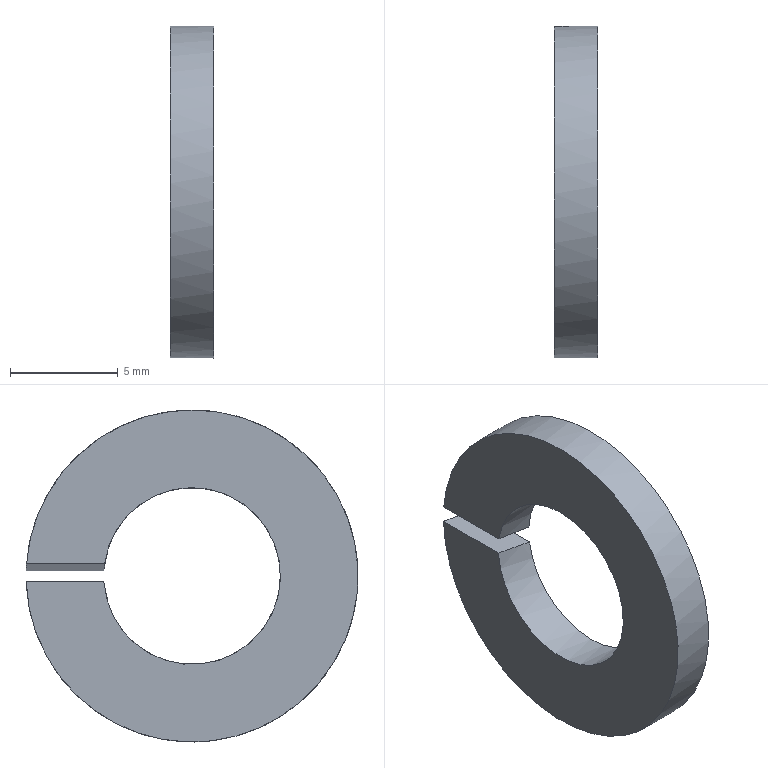Part | NX | features 5003_305_SLW8 2 | 1 solid | 6 faces | box 2 x 15.396 x 15.4 mm | volume 260.927 mm3 | plane 4 | cylinder 2 | commonest cylinder face diameters 8.2 x1 15.4 x1
STEP:
#1=CARTESIAN_POINT('',(383.29,-14.804,-169.49));
#2=VERTEX_POINT('',#1);
#3=CARTESIAN_POINT('',(383.29,-18.407,-169.49));
#4=VERTEX_POINT('',#3);
#5=CARTESIAN_POINT('',(383.29,-14.8,-169.49));
#6=DIRECTION('',(0.,-1.,0.));
#7=VECTOR('',#6,1000.);
#8=LINE('',#5,#7);
#9=EDGE_CURVE('',#2,#4,#8,.T.);
#10=ORIENTED_EDGE('',*,*,#9,.F.);
#11=CARTESIAN_POINT('',(383.29,-14.823,-168.66));
#12=VERTEX_POINT('',#11);
#13=CARTESIAN_POINT('',(383.29,-22.5,-169.25));
#14=DIRECTION('',(-1.,0.,0.));
#15=DIRECTION('',(0.,1.,0.));
#16=AXIS2_PLACEMENT_3D('',#13,#14,#15);
#17=CIRCLE('',#16,7.7);
#18=EDGE_CURVE('',#2,#12,#17,.T.);
#19=ORIENTED_EDGE('',*,*,#18,.T.);
#20=CARTESIAN_POINT('',(383.29,-18.443,-168.66));
#21=VERTEX_POINT('',#20);
#22=CARTESIAN_POINT('',(383.29,-14.8,-168.66));
#23=DIRECTION('',(0.,-1.,0.));
#24=VECTOR('',#23,1000.);
#25=LINE('',#22,#24);
#26=EDGE_CURVE('',#12,#21,#25,.T.);
#27=ORIENTED_EDGE('',*,*,#26,.T.);
#28=CARTESIAN_POINT('',(383.29,-22.5,-169.25));
#29=DIRECTION('',(-1.,0.,0.));
#30=DIRECTION('',(0.,1.,0.));
#31=AXIS2_PLACEMENT_3D('',#28,#29,#30);
#32=CIRCLE('',#31,4.1);
#33=EDGE_CURVE('',#4,#21,#32,.T.);
#34=ORIENTED_EDGE('',*,*,#33,.F.);
#35=EDGE_LOOP('',(#10,#19,#27,#34));
#36=FACE_BOUND('',#35,.T.);
#37=CARTESIAN_POINT('',(383.29,-22.5,-173.35));
#38=DIRECTION('',(1.,0.,0.));
#39=DIRECTION('',(0.,-1.,0.));
#40=AXIS2_PLACEMENT_3D('',#37,#38,#39);
#41=PLANE('',#40);
#42=ADVANCED_FACE('',(#36),#41,.F.);
#43=CARTESIAN_POINT('',(385.29,-14.823,-169.84));
#44=VERTEX_POINT('',#43);
#45=CARTESIAN_POINT('',(381.919,-22.5,-169.25));
#46=DIRECTION('',(0.1724,0.,0.985));
#47=DIRECTION('',(-0.985,0.,0.1724));
#48=AXIS2_PLACEMENT_3D('',#45,#46,#47);
#49=ELLIPSE('',#48,44.669,7.7);
#50=EDGE_CURVE('',#44,#2,#49,.T.);
#51=ORIENTED_EDGE('',*,*,#50,.F.);
#52=CARTESIAN_POINT('',(385.29,-14.804,-169.01));
#53=VERTEX_POINT('',#52);
#54=CARTESIAN_POINT('',(385.29,-22.5,-169.25));
#55=DIRECTION('',(-1.,0.,0.));
#56=DIRECTION('',(0.,1.,0.));
#57=AXIS2_PLACEMENT_3D('',#54,#55,#56);
#58=CIRCLE('',#57,7.7);
#59=EDGE_CURVE('',#44,#53,#58,.T.);
#60=ORIENTED_EDGE('',*,*,#59,.T.);
#61=CARTESIAN_POINT('',(386.662,-22.5,-169.25));
#62=DIRECTION('',(-0.1724,0.,-0.985));
#63=DIRECTION('',(-0.985,0.,0.1724));
#64=AXIS2_PLACEMENT_3D('',#61,#62,#63);
#65=ELLIPSE('',#64,44.669,7.7);
#66=EDGE_CURVE('',#12,#53,#65,.T.);
#67=ORIENTED_EDGE('',*,*,#66,.F.);
#68=ORIENTED_EDGE('',*,*,#18,.F.);
#69=EDGE_LOOP('',(#51,#60,#67,#68));
#70=FACE_BOUND('',#69,.T.);
#71=CARTESIAN_POINT('',(383.29,-22.5,-169.25));
#72=DIRECTION('',(-1.,0.,0.));
#73=DIRECTION('',(0.,1.,0.));
#74=AXIS2_PLACEMENT_3D('',#71,#72,#73);
#75=CYLINDRICAL_SURFACE('',#74,7.7);
#76=ADVANCED_FACE('',(#70),#75,.T.);
#77=CARTESIAN_POINT('',(385.29,-18.443,-169.84));
#78=VERTEX_POINT('',#77);
#79=CARTESIAN_POINT('',(385.29,-14.8,-169.84));
#80=DIRECTION('',(0.,-1.,0.));
#81=VECTOR('',#80,1000.);
#82=LINE('',#79,#81);
#83=EDGE_CURVE('',#44,#78,#82,.T.);
#84=ORIENTED_EDGE('',*,*,#83,.T.);
#85=CARTESIAN_POINT('',(385.29,-18.407,-169.01));
#86=VERTEX_POINT('',#85);
#87=CARTESIAN_POINT('',(385.29,-22.5,-169.25));
#88=DIRECTION('',(-1.,0.,0.));
#89=DIRECTION('',(0.,1.,0.));
#90=AXIS2_PLACEMENT_3D('',#87,#88,#89);
#91=CIRCLE('',#90,4.1);
#92=EDGE_CURVE('',#78,#86,#91,.T.);
#93=ORIENTED_EDGE('',*,*,#92,.T.);
#94=CARTESIAN_POINT('',(385.29,-14.8,-169.01));
#95=DIRECTION('',(0.,-1.,0.));
#96=VECTOR('',#95,1000.);
#97=LINE('',#94,#96);
#98=EDGE_CURVE('',#53,#86,#97,.T.);
#99=ORIENTED_EDGE('',*,*,#98,.F.);
#100=ORIENTED_EDGE('',*,*,#59,.F.);
#101=EDGE_LOOP('',(#84,#93,#99,#100));
#102=FACE_BOUND('',#101,.T.);
#103=CARTESIAN_POINT('',(385.29,-22.5,-173.35));
#104=DIRECTION('',(-1.,0.,0.));
#105=DIRECTION('',(0.,1.,0.));
#106=AXIS2_PLACEMENT_3D('',#103,#104,#105);
#107=PLANE('',#106);
#108=ADVANCED_FACE('',(#102),#107,.F.);
#109=CARTESIAN_POINT('',(381.919,-22.5,-169.25));
#110=DIRECTION('',(0.1724,0.,0.985));
#111=DIRECTION('',(-0.985,0.,0.1724));
#112=AXIS2_PLACEMENT_3D('',#109,#110,#111);
#113=ELLIPSE('',#112,23.785,4.1);
#114=EDGE_CURVE('',#4,#78,#113,.F.);
#115=ORIENTED_EDGE('',*,*,#114,.F.);
#116=ORIENTED_EDGE('',*,*,#33,.T.);
#117=CARTESIAN_POINT('',(386.662,-22.5,-169.25));
#118=DIRECTION('',(-0.1724,0.,-0.985));
#119=DIRECTION('',(-0.985,0.,0.1724));
#120=AXIS2_PLACEMENT_3D('',#117,#118,#119);
#121=ELLIPSE('',#120,23.785,4.1);
#122=EDGE_CURVE('',#86,#21,#121,.F.);
#123=ORIENTED_EDGE('',*,*,#122,.F.);
#124=ORIENTED_EDGE('',*,*,#92,.F.);
#125=EDGE_LOOP('',(#115,#116,#123,#124));
#126=FACE_BOUND('',#125,.T.);
#127=CARTESIAN_POINT('',(383.29,-22.5,-169.25));
#128=DIRECTION('',(-1.,0.,0.));
#129=DIRECTION('',(0.,1.,0.));
#130=AXIS2_PLACEMENT_3D('',#127,#128,#129);
#131=CYLINDRICAL_SURFACE('',#130,4.1);
#132=ADVANCED_FACE('',(#126),#131,.F.);
#133=ORIENTED_EDGE('',*,*,#66,.T.);
#134=ORIENTED_EDGE('',*,*,#98,.T.);
#135=ORIENTED_EDGE('',*,*,#122,.T.);
#136=ORIENTED_EDGE('',*,*,#26,.F.);
#137=EDGE_LOOP('',(#133,#134,#135,#136));
#138=FACE_BOUND('',#137,.T.);
#139=CARTESIAN_POINT('',(383.29,-14.8,-168.66));
#140=DIRECTION('',(-0.1724,0.,-0.985));
#141=DIRECTION('',(-0.985,0.,0.1724));
#142=AXIS2_PLACEMENT_3D('',#139,#140,#141);
#143=PLANE('',#142);
#144=ADVANCED_FACE('',(#138),#143,.T.);
#145=ORIENTED_EDGE('',*,*,#50,.T.);
#146=ORIENTED_EDGE('',*,*,#9,.T.);
#147=ORIENTED_EDGE('',*,*,#114,.T.);
#148=ORIENTED_EDGE('',*,*,#83,.F.);
#149=EDGE_LOOP('',(#145,#146,#147,#148));
#150=FACE_BOUND('',#149,.T.);
#151=CARTESIAN_POINT('',(385.29,-14.8,-169.84));
#152=DIRECTION('',(0.1724,0.,0.985));
#153=DIRECTION('',(0.985,0.,-0.1724));
#154=AXIS2_PLACEMENT_3D('',#151,#152,#153);
#155=PLANE('',#154);
#156=ADVANCED_FACE('',(#150),#155,.T.);
#157=CLOSED_SHELL('',(#42,#76,#108,#132,#144,#156));
#158=MANIFOLD_SOLID_BREP('',#157);
#159=(LENGTH_UNIT()NAMED_UNIT(*)SI_UNIT(.MILLI.,.METRE.));
#160=UNCERTAINTY_MEASURE_WITH_UNIT(LENGTH_MEASURE(0.00001),#159,'','');
#161=(NAMED_UNIT(*)PLANE_ANGLE_UNIT()SI_UNIT($,.RADIAN.));
#162=(NAMED_UNIT(*)SI_UNIT($,.STERADIAN.)SOLID_ANGLE_UNIT());
#163=(GEOMETRIC_REPRESENTATION_CONTEXT(3)GLOBAL_UNCERTAINTY_ASSIGNED_CONTEXT((#160))GLOBAL_UNIT_ASSIGNED_CONTEXT((#159,#161,#162))REPRESENTATION_CONTEXT('',''));
#164=ADVANCED_BREP_SHAPE_REPRESENTATION('',(#158),#163);